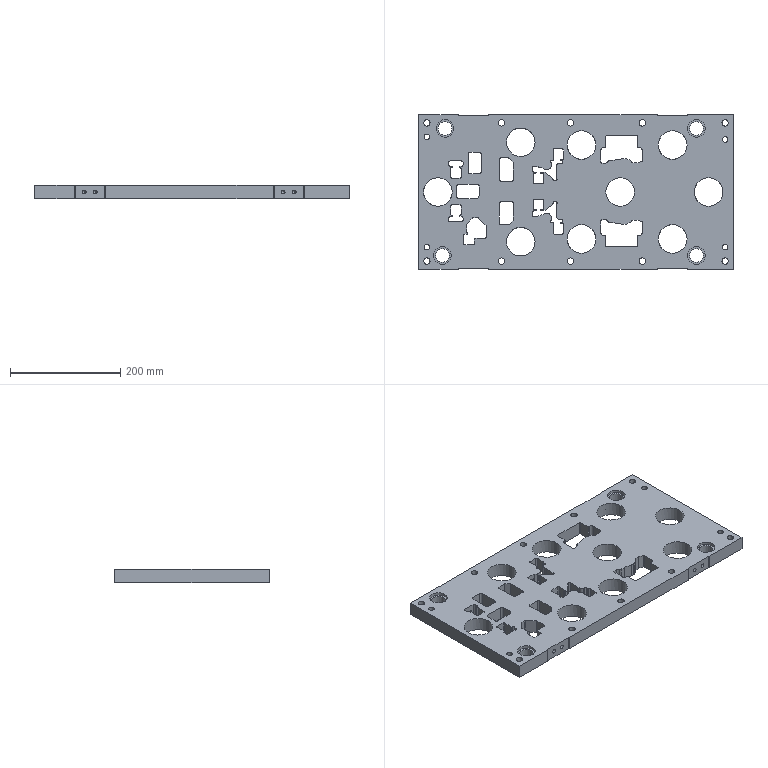Part | NX | features PH-1 2 | 1 solid | 373 faces | box 570 x 280 x 25 mm | volume 2996818 mm3 | cylinder 165 | plane 154 | spline 46 | cone 8 | commonest cylinder face diameters 4 x51 1 x27 6 x21 10 x10 11.5 x10 18 x10